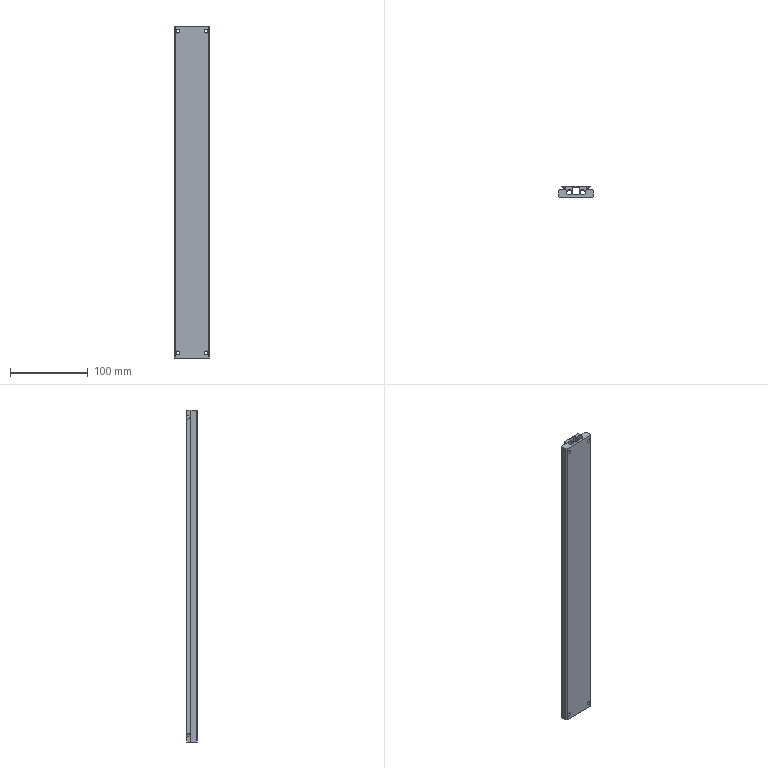Part | STEP file | P193368_BVP_HMPL_16_160 | 1 solid | 55 faces | box 45 x 14 x 426.6 mm | volume 169280 mm3 | cylinder 29 | plane 26 | commonest cylinder face diameters 4.5 x8 8 x8 7 x4 10 x4 0.5 x3 2.4 x2